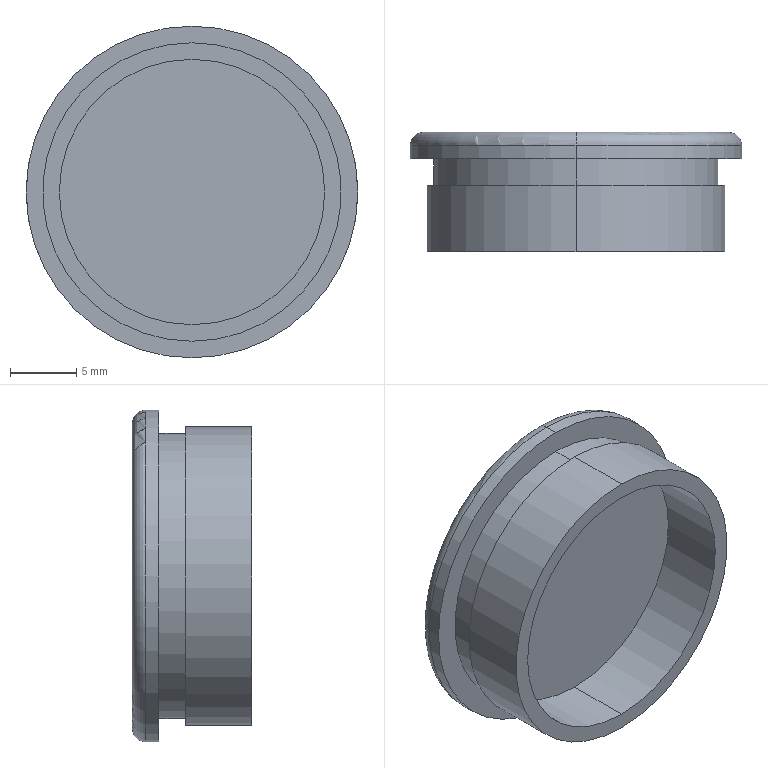Part | STEP file | A22NE-A-401 | 1 solid | 15 faces | box 25 x 9 x 25 mm | volume 2109 mm3 | cylinder 8 | plane 5 | torus 2 | commonest cylinder face diameters 20 x2 21.5 x2 22.5 x2 25 x2
STEP:
#1=CARTESIAN_POINT('',(0.,8.,-12.5));
#2=VERTEX_POINT('',#1);
#3=CARTESIAN_POINT('',(0.,8.,12.5));
#4=VERTEX_POINT('',#3);
#5=CARTESIAN_POINT('',(0.,8.,0.));
#6=DIRECTION('',(0.,-1.,0.));
#7=DIRECTION('',(0.,0.,1.));
#8=AXIS2_PLACEMENT_3D('',#5,#6,#7);
#9=CIRCLE('',#8,12.5);
#10=EDGE_CURVE('',#2,#4,#9,.T.);
#11=ORIENTED_EDGE('',*,*,#10,.F.);
#12=CARTESIAN_POINT('',(0.,9.,-11.5));
#13=VERTEX_POINT('',#12);
#14=CARTESIAN_POINT('',(0.,8.,-11.5));
#15=DIRECTION('',(1.,0.,0.));
#16=DIRECTION('',(0.,0.,-1.));
#17=AXIS2_PLACEMENT_3D('',#14,#15,#16);
#18=CIRCLE('',#17,1.);
#19=EDGE_CURVE('',#2,#13,#18,.T.);
#20=ORIENTED_EDGE('',*,*,#19,.T.);
#21=CARTESIAN_POINT('',(0.,9.,11.5));
#22=VERTEX_POINT('',#21);
#23=CARTESIAN_POINT('',(0.,9.,0.));
#24=DIRECTION('',(0.,1.,0.));
#25=DIRECTION('',(0.,0.,1.));
#26=AXIS2_PLACEMENT_3D('',#23,#24,#25);
#27=CIRCLE('',#26,11.5);
#28=EDGE_CURVE('',#22,#13,#27,.T.);
#29=ORIENTED_EDGE('',*,*,#28,.F.);
#30=CARTESIAN_POINT('',(0.,8.,11.5));
#31=DIRECTION('',(-1.,0.,0.));
#32=DIRECTION('',(0.,0.,1.));
#33=AXIS2_PLACEMENT_3D('',#30,#31,#32);
#34=CIRCLE('',#33,1.);
#35=EDGE_CURVE('',#4,#22,#34,.T.);
#36=ORIENTED_EDGE('',*,*,#35,.F.);
#37=EDGE_LOOP('',(#11,#20,#29,#36));
#38=FACE_OUTER_BOUND('',#37,.T.);
#39=CARTESIAN_POINT('',(0.,8.,0.));
#40=DIRECTION('',(0.,1.,0.));
#41=DIRECTION('',(0.,0.,1.));
#42=AXIS2_PLACEMENT_3D('',#39,#40,#41);
#43=TOROIDAL_SURFACE('',#42,11.5,1.);
#44=ADVANCED_FACE('',(#38),#43,.T.);
#45=CARTESIAN_POINT('',(0.,5.,10.));
#46=VERTEX_POINT('',#45);
#47=CARTESIAN_POINT('',(0.,5.,-10.));
#48=VERTEX_POINT('',#47);
#49=CARTESIAN_POINT('',(0.,5.,0.));
#50=DIRECTION('',(0.,-1.,0.));
#51=DIRECTION('',(0.,0.,-1.));
#52=AXIS2_PLACEMENT_3D('',#49,#50,#51);
#53=CIRCLE('',#52,10.);
#54=EDGE_CURVE('',#46,#48,#53,.T.);
#55=ORIENTED_EDGE('',*,*,#54,.F.);
#56=CARTESIAN_POINT('',(0.,0.,10.));
#57=VERTEX_POINT('',#56);
#58=CARTESIAN_POINT('',(0.,5.,10.));
#59=DIRECTION('',(0.,-1.,0.));
#60=VECTOR('',#59,1000.);
#61=LINE('',#58,#60);
#62=EDGE_CURVE('',#46,#57,#61,.T.);
#63=ORIENTED_EDGE('',*,*,#62,.T.);
#64=CARTESIAN_POINT('',(0.,0.,-10.));
#65=VERTEX_POINT('',#64);
#66=CARTESIAN_POINT('',(0.,0.,0.));
#67=DIRECTION('',(0.,-1.,0.));
#68=DIRECTION('',(0.,0.,-1.));
#69=AXIS2_PLACEMENT_3D('',#66,#67,#68);
#70=CIRCLE('',#69,10.);
#71=EDGE_CURVE('',#57,#65,#70,.T.);
#72=ORIENTED_EDGE('',*,*,#71,.T.);
#73=CARTESIAN_POINT('',(0.,5.,-10.));
#74=DIRECTION('',(0.,-1.,0.));
#75=VECTOR('',#74,1000.);
#76=LINE('',#73,#75);
#77=EDGE_CURVE('',#48,#65,#76,.T.);
#78=ORIENTED_EDGE('',*,*,#77,.F.);
#79=EDGE_LOOP('',(#55,#63,#72,#78));
#80=FACE_OUTER_BOUND('',#79,.T.);
#81=CARTESIAN_POINT('',(0.,5.,0.));
#82=DIRECTION('',(0.,-1.,0.));
#83=DIRECTION('',(0.,0.,-1.));
#84=AXIS2_PLACEMENT_3D('',#81,#82,#83);
#85=CYLINDRICAL_SURFACE('',#84,10.);
#86=ADVANCED_FACE('',(#80),#85,.F.);
#87=ORIENTED_EDGE('',*,*,#10,.T.);
#88=CARTESIAN_POINT('',(0.,7.,12.5));
#89=VERTEX_POINT('',#88);
#90=CARTESIAN_POINT('',(0.,0.,12.5));
#91=DIRECTION('',(0.,-1.,0.));
#92=VECTOR('',#91,1000.);
#93=LINE('',#90,#92);
#94=EDGE_CURVE('',#4,#89,#93,.T.);
#95=ORIENTED_EDGE('',*,*,#94,.T.);
#96=CARTESIAN_POINT('',(0.,7.,-12.5));
#97=VERTEX_POINT('',#96);
#98=CARTESIAN_POINT('',(0.,7.,0.));
#99=DIRECTION('',(0.,-1.,0.));
#100=DIRECTION('',(0.,0.,-1.));
#101=AXIS2_PLACEMENT_3D('',#98,#99,#100);
#102=CIRCLE('',#101,12.5);
#103=EDGE_CURVE('',#97,#89,#102,.T.);
#104=ORIENTED_EDGE('',*,*,#103,.F.);
#105=CARTESIAN_POINT('',(0.,0.,-12.5));
#106=DIRECTION('',(0.,-1.,0.));
#107=VECTOR('',#106,1000.);
#108=LINE('',#105,#107);
#109=EDGE_CURVE('',#2,#97,#108,.T.);
#110=ORIENTED_EDGE('',*,*,#109,.F.);
#111=EDGE_LOOP('',(#87,#95,#104,#110));
#112=FACE_OUTER_BOUND('',#111,.T.);
#113=CARTESIAN_POINT('',(0.,0.,0.));
#114=DIRECTION('',(0.,-1.,0.));
#115=DIRECTION('',(0.,0.,-1.));
#116=AXIS2_PLACEMENT_3D('',#113,#114,#115);
#117=CYLINDRICAL_SURFACE('',#116,12.5);
#118=ADVANCED_FACE('',(#112),#117,.T.);
#119=CARTESIAN_POINT('',(0.,7.,-10.75));
#120=VERTEX_POINT('',#119);
#121=CARTESIAN_POINT('',(0.,7.,10.75));
#122=VERTEX_POINT('',#121);
#123=CARTESIAN_POINT('',(0.,7.,0.));
#124=DIRECTION('',(0.,-1.,0.));
#125=DIRECTION('',(0.,0.,-1.));
#126=AXIS2_PLACEMENT_3D('',#123,#124,#125);
#127=CIRCLE('',#126,10.75);
#128=EDGE_CURVE('',#120,#122,#127,.T.);
#129=ORIENTED_EDGE('',*,*,#128,.T.);
#130=CARTESIAN_POINT('',(0.,5.,10.75));
#131=VERTEX_POINT('',#130);
#132=CARTESIAN_POINT('',(0.,0.,10.75));
#133=DIRECTION('',(0.,-1.,0.));
#134=VECTOR('',#133,1000.);
#135=LINE('',#132,#134);
#136=EDGE_CURVE('',#122,#131,#135,.T.);
#137=ORIENTED_EDGE('',*,*,#136,.T.);
#138=CARTESIAN_POINT('',(0.,5.,-10.75));
#139=VERTEX_POINT('',#138);
#140=CARTESIAN_POINT('',(0.,5.,0.));
#141=DIRECTION('',(0.,-1.,0.));
#142=DIRECTION('',(0.,0.,-1.));
#143=AXIS2_PLACEMENT_3D('',#140,#141,#142);
#144=CIRCLE('',#143,10.75);
#145=EDGE_CURVE('',#139,#131,#144,.T.);
#146=ORIENTED_EDGE('',*,*,#145,.F.);
#147=CARTESIAN_POINT('',(0.,0.,-10.75));
#148=DIRECTION('',(0.,-1.,0.));
#149=VECTOR('',#148,1000.);
#150=LINE('',#147,#149);
#151=EDGE_CURVE('',#120,#139,#150,.T.);
#152=ORIENTED_EDGE('',*,*,#151,.F.);
#153=EDGE_LOOP('',(#129,#137,#146,#152));
#154=FACE_OUTER_BOUND('',#153,.T.);
#155=CARTESIAN_POINT('',(0.,0.,0.));
#156=DIRECTION('',(0.,-1.,0.));
#157=DIRECTION('',(0.,0.,-1.));
#158=AXIS2_PLACEMENT_3D('',#155,#156,#157);
#159=CYLINDRICAL_SURFACE('',#158,10.75);
#160=ADVANCED_FACE('',(#154),#159,.T.);
#161=CARTESIAN_POINT('',(0.,5.,-11.25));
#162=VERTEX_POINT('',#161);
#163=CARTESIAN_POINT('',(0.,5.,11.25));
#164=VERTEX_POINT('',#163);
#165=CARTESIAN_POINT('',(0.,5.,0.));
#166=DIRECTION('',(0.,-1.,0.));
#167=DIRECTION('',(0.,0.,-1.));
#168=AXIS2_PLACEMENT_3D('',#165,#166,#167);
#169=CIRCLE('',#168,11.25);
#170=EDGE_CURVE('',#162,#164,#169,.T.);
#171=ORIENTED_EDGE('',*,*,#170,.T.);
#172=CARTESIAN_POINT('',(0.,0.,11.25));
#173=VERTEX_POINT('',#172);
#174=CARTESIAN_POINT('',(0.,0.,11.25));
#175=DIRECTION('',(0.,-1.,0.));
#176=VECTOR('',#175,1000.);
#177=LINE('',#174,#176);
#178=EDGE_CURVE('',#164,#173,#177,.T.);
#179=ORIENTED_EDGE('',*,*,#178,.T.);
#180=CARTESIAN_POINT('',(0.,0.,-11.25));
#181=VERTEX_POINT('',#180);
#182=CARTESIAN_POINT('',(0.,0.,0.));
#183=DIRECTION('',(0.,-1.,0.));
#184=DIRECTION('',(0.,0.,-1.));
#185=AXIS2_PLACEMENT_3D('',#182,#183,#184);
#186=CIRCLE('',#185,11.25);
#187=EDGE_CURVE('',#181,#173,#186,.T.);
#188=ORIENTED_EDGE('',*,*,#187,.F.);
#189=CARTESIAN_POINT('',(0.,0.,-11.25));
#190=DIRECTION('',(0.,-1.,0.));
#191=VECTOR('',#190,1000.);
#192=LINE('',#189,#191);
#193=EDGE_CURVE('',#162,#181,#192,.T.);
#194=ORIENTED_EDGE('',*,*,#193,.F.);
#195=EDGE_LOOP('',(#171,#179,#188,#194));
#196=FACE_OUTER_BOUND('',#195,.T.);
#197=CARTESIAN_POINT('',(0.,0.,0.));
#198=DIRECTION('',(0.,-1.,0.));
#199=DIRECTION('',(0.,0.,-1.));
#200=AXIS2_PLACEMENT_3D('',#197,#198,#199);
#201=CYLINDRICAL_SURFACE('',#200,11.25);
#202=ADVANCED_FACE('',(#196),#201,.T.);
#203=CARTESIAN_POINT('',(0.,0.,0.));
#204=DIRECTION('',(0.,-1.,0.));
#205=DIRECTION('',(0.,0.,-1.));
#206=AXIS2_PLACEMENT_3D('',#203,#204,#205);
#207=CIRCLE('',#206,10.);
#208=EDGE_CURVE('',#65,#57,#207,.T.);
#209=ORIENTED_EDGE('',*,*,#208,.F.);
#210=ORIENTED_EDGE('',*,*,#71,.F.);
#211=EDGE_LOOP('',(#209,#210));
#212=FACE_BOUND('',#211,.T.);
#213=ORIENTED_EDGE('',*,*,#187,.T.);
#214=CARTESIAN_POINT('',(0.,0.,0.));
#215=DIRECTION('',(0.,-1.,0.));
#216=DIRECTION('',(0.,0.,-1.));
#217=AXIS2_PLACEMENT_3D('',#214,#215,#216);
#218=CIRCLE('',#217,11.25);
#219=EDGE_CURVE('',#173,#181,#218,.T.);
#220=ORIENTED_EDGE('',*,*,#219,.T.);
#221=EDGE_LOOP('',(#213,#220));
#222=FACE_OUTER_BOUND('',#221,.T.);
#223=CARTESIAN_POINT('',(0.,0.,0.));
#224=DIRECTION('',(0.,-1.,0.));
#225=DIRECTION('',(0.,0.,-1.));
#226=AXIS2_PLACEMENT_3D('',#223,#224,#225);
#227=PLANE('',#226);
#228=ADVANCED_FACE('',(#212,#222),#227,.T.);
#229=ORIENTED_EDGE('',*,*,#178,.F.);
#230=CARTESIAN_POINT('',(0.,5.,0.));
#231=DIRECTION('',(0.,-1.,0.));
#232=DIRECTION('',(0.,0.,-1.));
#233=AXIS2_PLACEMENT_3D('',#230,#231,#232);
#234=CIRCLE('',#233,11.25);
#235=EDGE_CURVE('',#164,#162,#234,.T.);
#236=ORIENTED_EDGE('',*,*,#235,.T.);
#237=ORIENTED_EDGE('',*,*,#193,.T.);
#238=ORIENTED_EDGE('',*,*,#219,.F.);
#239=EDGE_LOOP('',(#229,#236,#237,#238));
#240=FACE_OUTER_BOUND('',#239,.T.);
#241=CARTESIAN_POINT('',(0.,0.,0.));
#242=DIRECTION('',(0.,-1.,0.));
#243=DIRECTION('',(0.,0.,-1.));
#244=AXIS2_PLACEMENT_3D('',#241,#242,#243);
#245=CYLINDRICAL_SURFACE('',#244,11.25);
#246=ADVANCED_FACE('',(#240),#245,.T.);
#247=ORIENTED_EDGE('',*,*,#145,.T.);
#248=CARTESIAN_POINT('',(0.,5.,0.));
#249=DIRECTION('',(0.,-1.,0.));
#250=DIRECTION('',(0.,0.,-1.));
#251=AXIS2_PLACEMENT_3D('',#248,#249,#250);
#252=CIRCLE('',#251,10.75);
#253=EDGE_CURVE('',#131,#139,#252,.T.);
#254=ORIENTED_EDGE('',*,*,#253,.T.);
#255=EDGE_LOOP('',(#247,#254));
#256=FACE_BOUND('',#255,.T.);
#257=ORIENTED_EDGE('',*,*,#170,.F.);
#258=ORIENTED_EDGE('',*,*,#235,.F.);
#259=EDGE_LOOP('',(#257,#258));
#260=FACE_OUTER_BOUND('',#259,.T.);
#261=CARTESIAN_POINT('',(10.75,5.,0.));
#262=DIRECTION('',(0.,1.,0.));
#263=DIRECTION('',(0.,0.,1.));
#264=AXIS2_PLACEMENT_3D('',#261,#262,#263);
#265=PLANE('',#264);
#266=ADVANCED_FACE('',(#256,#260),#265,.T.);
#267=ORIENTED_EDGE('',*,*,#136,.F.);
#268=CARTESIAN_POINT('',(0.,7.,0.));
#269=DIRECTION('',(0.,-1.,0.));
#270=DIRECTION('',(0.,0.,-1.));
#271=AXIS2_PLACEMENT_3D('',#268,#269,#270);
#272=CIRCLE('',#271,10.75);
#273=EDGE_CURVE('',#122,#120,#272,.T.);
#274=ORIENTED_EDGE('',*,*,#273,.T.);
#275=ORIENTED_EDGE('',*,*,#151,.T.);
#276=ORIENTED_EDGE('',*,*,#253,.F.);
#277=EDGE_LOOP('',(#267,#274,#275,#276));
#278=FACE_OUTER_BOUND('',#277,.T.);
#279=CARTESIAN_POINT('',(0.,0.,0.));
#280=DIRECTION('',(0.,-1.,0.));
#281=DIRECTION('',(0.,0.,-1.));
#282=AXIS2_PLACEMENT_3D('',#279,#280,#281);
#283=CYLINDRICAL_SURFACE('',#282,10.75);
#284=ADVANCED_FACE('',(#278),#283,.T.);
#285=ORIENTED_EDGE('',*,*,#103,.T.);
#286=CARTESIAN_POINT('',(0.,7.,0.));
#287=DIRECTION('',(0.,-1.,0.));
#288=DIRECTION('',(0.,0.,-1.));
#289=AXIS2_PLACEMENT_3D('',#286,#287,#288);
#290=CIRCLE('',#289,12.5);
#291=EDGE_CURVE('',#89,#97,#290,.T.);
#292=ORIENTED_EDGE('',*,*,#291,.T.);
#293=EDGE_LOOP('',(#285,#292));
#294=FACE_OUTER_BOUND('',#293,.T.);
#295=ORIENTED_EDGE('',*,*,#128,.F.);
#296=ORIENTED_EDGE('',*,*,#273,.F.);
#297=EDGE_LOOP('',(#295,#296));
#298=FACE_BOUND('',#297,.T.);
#299=CARTESIAN_POINT('',(10.75,7.,0.));
#300=DIRECTION('',(0.,-1.,0.));
#301=DIRECTION('',(0.,0.,-1.));
#302=AXIS2_PLACEMENT_3D('',#299,#300,#301);
#303=PLANE('',#302);
#304=ADVANCED_FACE('',(#294,#298),#303,.T.);
#305=ORIENTED_EDGE('',*,*,#94,.F.);
#306=CARTESIAN_POINT('',(0.,8.,0.));
#307=DIRECTION('',(0.,-1.,0.));
#308=DIRECTION('',(0.,0.,1.));
#309=AXIS2_PLACEMENT_3D('',#306,#307,#308);
#310=CIRCLE('',#309,12.5);
#311=EDGE_CURVE('',#4,#2,#310,.T.);
#312=ORIENTED_EDGE('',*,*,#311,.T.);
#313=ORIENTED_EDGE('',*,*,#109,.T.);
#314=ORIENTED_EDGE('',*,*,#291,.F.);
#315=EDGE_LOOP('',(#305,#312,#313,#314));
#316=FACE_OUTER_BOUND('',#315,.T.);
#317=CARTESIAN_POINT('',(0.,0.,0.));
#318=DIRECTION('',(0.,-1.,0.));
#319=DIRECTION('',(0.,0.,-1.));
#320=AXIS2_PLACEMENT_3D('',#317,#318,#319);
#321=CYLINDRICAL_SURFACE('',#320,12.5);
#322=ADVANCED_FACE('',(#316),#321,.T.);
#323=ORIENTED_EDGE('',*,*,#28,.T.);
#324=CARTESIAN_POINT('',(0.,9.,0.));
#325=DIRECTION('',(0.,1.,0.));
#326=DIRECTION('',(0.,0.,1.));
#327=AXIS2_PLACEMENT_3D('',#324,#325,#326);
#328=CIRCLE('',#327,11.5);
#329=EDGE_CURVE('',#13,#22,#328,.T.);
#330=ORIENTED_EDGE('',*,*,#329,.T.);
#331=EDGE_LOOP('',(#323,#330));
#332=FACE_OUTER_BOUND('',#331,.T.);
#333=CARTESIAN_POINT('',(12.5,9.,0.));
#334=DIRECTION('',(0.,1.,0.));
#335=DIRECTION('',(0.,0.,1.));
#336=AXIS2_PLACEMENT_3D('',#333,#334,#335);
#337=PLANE('',#336);
#338=ADVANCED_FACE('',(#332),#337,.T.);
#339=ORIENTED_EDGE('',*,*,#62,.F.);
#340=CARTESIAN_POINT('',(0.,5.,0.));
#341=DIRECTION('',(0.,-1.,0.));
#342=DIRECTION('',(0.,0.,-1.));
#343=AXIS2_PLACEMENT_3D('',#340,#341,#342);
#344=CIRCLE('',#343,10.);
#345=EDGE_CURVE('',#48,#46,#344,.T.);
#346=ORIENTED_EDGE('',*,*,#345,.F.);
#347=ORIENTED_EDGE('',*,*,#77,.T.);
#348=ORIENTED_EDGE('',*,*,#208,.T.);
#349=EDGE_LOOP('',(#339,#346,#347,#348));
#350=FACE_OUTER_BOUND('',#349,.T.);
#351=CARTESIAN_POINT('',(0.,5.,0.));
#352=DIRECTION('',(0.,-1.,0.));
#353=DIRECTION('',(0.,0.,-1.));
#354=AXIS2_PLACEMENT_3D('',#351,#352,#353);
#355=CYLINDRICAL_SURFACE('',#354,10.);
#356=ADVANCED_FACE('',(#350),#355,.F.);
#357=ORIENTED_EDGE('',*,*,#345,.T.);
#358=ORIENTED_EDGE('',*,*,#54,.T.);
#359=EDGE_LOOP('',(#357,#358));
#360=FACE_OUTER_BOUND('',#359,.T.);
#361=CARTESIAN_POINT('',(0.,5.,0.));
#362=DIRECTION('',(0.,-1.,0.));
#363=DIRECTION('',(0.,0.,-1.));
#364=AXIS2_PLACEMENT_3D('',#361,#362,#363);
#365=PLANE('',#364);
#366=ADVANCED_FACE('',(#360),#365,.T.);
#367=ORIENTED_EDGE('',*,*,#19,.F.);
#368=ORIENTED_EDGE('',*,*,#311,.F.);
#369=ORIENTED_EDGE('',*,*,#35,.T.);
#370=ORIENTED_EDGE('',*,*,#329,.F.);
#371=EDGE_LOOP('',(#367,#368,#369,#370));
#372=FACE_OUTER_BOUND('',#371,.T.);
#373=CARTESIAN_POINT('',(0.,8.,0.));
#374=DIRECTION('',(0.,1.,0.));
#375=DIRECTION('',(0.,0.,1.));
#376=AXIS2_PLACEMENT_3D('',#373,#374,#375);
#377=TOROIDAL_SURFACE('',#376,11.5,1.);
#378=ADVANCED_FACE('',(#372),#377,.T.);
#379=CLOSED_SHELL('',(#44,#86,#118,#160,#202,#228,#246,#266,#284,#304,#322,#338,#356,#366,#378));
#380=MANIFOLD_SOLID_BREP('',#379);
#381=CARTESIAN_POINT('',(0.,0.,0.));
#382=DIRECTION('',(0.,0.,1.));
#383=DIRECTION('',(1.,0.,0.));
#384=AXIS2_PLACEMENT_3D('',#381,#382,#383);
#385=(LENGTH_UNIT()NAMED_UNIT(*)SI_UNIT(.MILLI.,.METRE.));
#386=UNCERTAINTY_MEASURE_WITH_UNIT(LENGTH_MEASURE(0.00001),#385,'','');
#387=(NAMED_UNIT(*)PLANE_ANGLE_UNIT()SI_UNIT($,.RADIAN.));
#388=(NAMED_UNIT(*)SI_UNIT($,.STERADIAN.)SOLID_ANGLE_UNIT());
#389=(GEOMETRIC_REPRESENTATION_CONTEXT(3)GLOBAL_UNCERTAINTY_ASSIGNED_CONTEXT((#386))GLOBAL_UNIT_ASSIGNED_CONTEXT((#385,#387,#388))REPRESENTATION_CONTEXT('',''));
#390=ADVANCED_BREP_SHAPE_REPRESENTATION('',(#380,#384),#389);